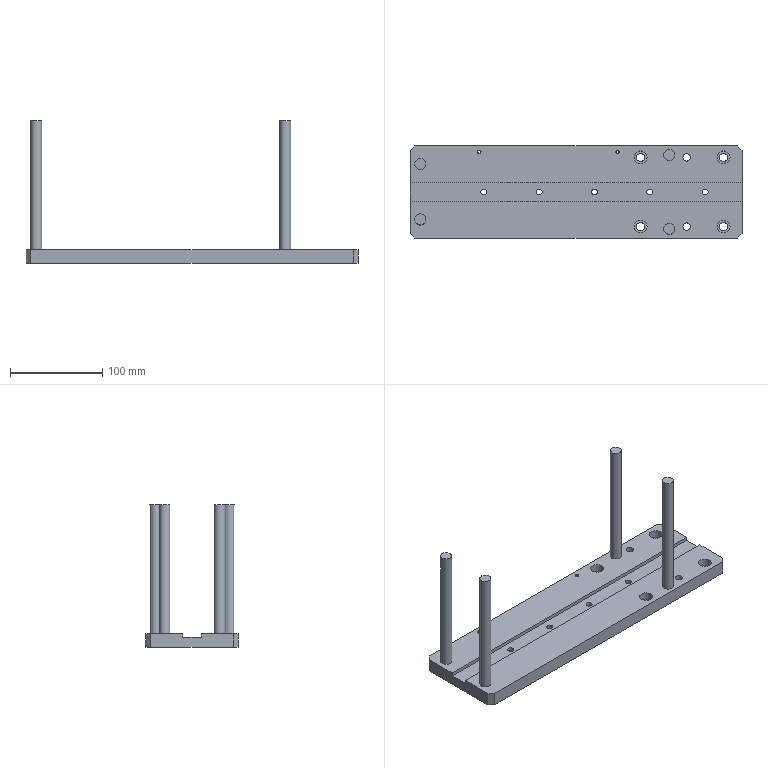Part | STEP file | Tube feed_id838_x_t | 1 solid | 65 faces | box 360 x 100 x 155 mm | volume 559892 mm3 | plane 31 | cylinder 30 | cone 4 | commonest cylinder face diameters 6.5 x7 10.5 x7 9 x4 12 x4 14 x4 3.3 x2